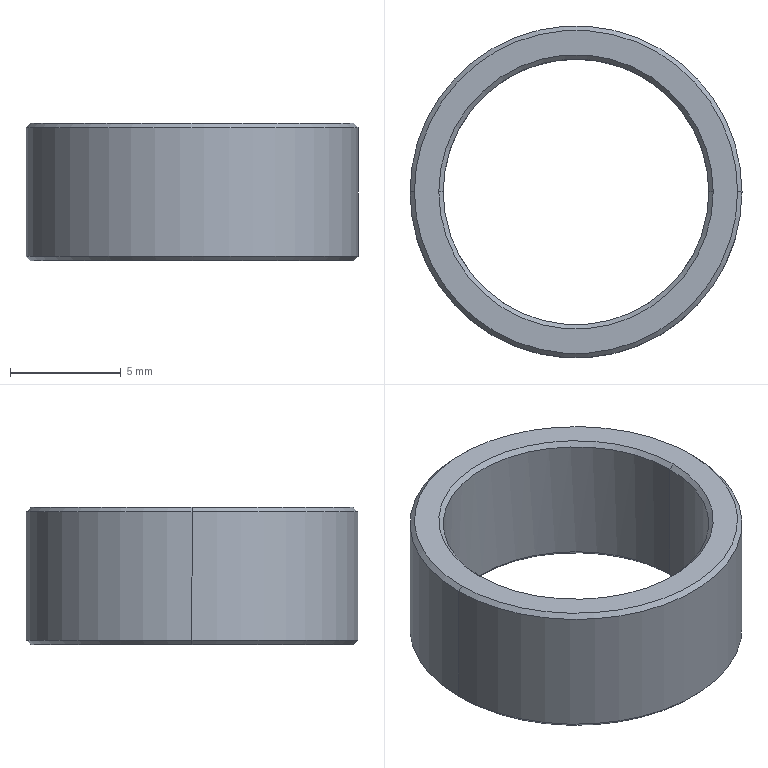Part | STEP file | 0243_002_FWSSM-D15-V12-T6.2 | 1 solid | 14 faces | box 15 x 15 x 6.2 mm | volume 391.034 mm3 | cone 8 | cylinder 4 | plane 2 | commonest cylinder face diameters 12 x2 15 x2
STEP:
#1=CARTESIAN_POINT('',(0.,0.,0.));
#2=DIRECTION('',(0.,0.,1.));
#3=DIRECTION('',(1.,0.,0.));
#4=AXIS2_PLACEMENT_3D('',#1,#2,#3);
#5=CARTESIAN_POINT('',(7.5,0.,-6.));
#6=VERTEX_POINT('',#5);
#7=CARTESIAN_POINT('',(-7.5,0.,-6.));
#8=VERTEX_POINT('',#7);
#9=CARTESIAN_POINT('',(0.,0.,-6.));
#10=DIRECTION('',(0.,0.,1.));
#11=DIRECTION('',(1.,0.,0.));
#12=AXIS2_PLACEMENT_3D('',#9,#10,#11);
#13=CIRCLE('',#12,7.5);
#14=CARTESIAN_POINT('',(0.,0.,-3.1));
#15=DIRECTION('',(0.,0.,1.));
#16=DIRECTION('',(1.,0.,0.));
#17=AXIS2_PLACEMENT_3D('',#14,#15,#16);
#18=CYLINDRICAL_SURFACE('',#17,7.5);
#19=CARTESIAN_POINT('',(0.,-2.9));
#20=DIRECTION('',(1.,0.));
#21=VECTOR('',#20,1.);
#22=LINE('',#19,#21);
#23=(GEOMETRIC_REPRESENTATION_CONTEXT(2)PARAMETRIC_REPRESENTATION_CONTEXT()REPRESENTATION_CONTEXT('',''));
#24=DEFINITIONAL_REPRESENTATION('',(#22),#23);
#25=PCURVE('',#18,#24);
#26=CARTESIAN_POINT('',(0.,0.,-6.));
#27=DIRECTION('',(0.,0.,1.));
#28=DIRECTION('',(1.,0.,0.));
#29=AXIS2_PLACEMENT_3D('',#26,#27,#28);
#30=CONICAL_SURFACE('',#29,7.5,0.7854);
#31=CARTESIAN_POINT('',(0.,0.));
#32=DIRECTION('',(1.,0.));
#33=VECTOR('',#32,1.);
#34=LINE('',#31,#33);
#35=(GEOMETRIC_REPRESENTATION_CONTEXT(2)PARAMETRIC_REPRESENTATION_CONTEXT()REPRESENTATION_CONTEXT('',''));
#36=DEFINITIONAL_REPRESENTATION('',(#34),#35);
#37=PCURVE('',#30,#36);
#38=SURFACE_CURVE('',#13,(#25,#37),.PCURVE_S1.);
#39=EDGE_CURVE('',#6,#8,#38,.T.);
#40=ORIENTED_EDGE('',*,*,#39,.T.);
#41=CARTESIAN_POINT('',(-7.5,0.,-0.2));
#42=VERTEX_POINT('',#41);
#43=CARTESIAN_POINT('',(-7.5,0.,-3.1));
#44=DIRECTION('',(0.,0.,1.));
#45=VECTOR('',#44,1.);
#46=LINE('',#43,#45);
#47=CARTESIAN_POINT('',(3.142,0.));
#48=DIRECTION('',(0.,1.));
#49=VECTOR('',#48,1.);
#50=LINE('',#47,#49);
#51=(GEOMETRIC_REPRESENTATION_CONTEXT(2)PARAMETRIC_REPRESENTATION_CONTEXT()REPRESENTATION_CONTEXT('',''));
#52=DEFINITIONAL_REPRESENTATION('',(#50),#51);
#53=PCURVE('',#18,#52);
#54=CARTESIAN_POINT('',(0.,0.,-3.1));
#55=DIRECTION('',(0.,0.,1.));
#56=DIRECTION('',(1.,0.,0.));
#57=AXIS2_PLACEMENT_3D('',#54,#55,#56);
#58=CYLINDRICAL_SURFACE('',#57,7.5);
#59=CARTESIAN_POINT('',(3.142,0.));
#60=DIRECTION('',(0.,1.));
#61=VECTOR('',#60,1.);
#62=LINE('',#59,#61);
#63=(GEOMETRIC_REPRESENTATION_CONTEXT(2)PARAMETRIC_REPRESENTATION_CONTEXT()REPRESENTATION_CONTEXT('',''));
#64=DEFINITIONAL_REPRESENTATION('',(#62),#63);
#65=PCURVE('',#58,#64);
#66=SURFACE_CURVE('',#46,(#53,#65),.PCURVE_S1.);
#67=EDGE_CURVE('',#8,#42,#66,.T.);
#68=ORIENTED_EDGE('',*,*,#67,.T.);
#69=CARTESIAN_POINT('',(7.5,0.,-0.2));
#70=VERTEX_POINT('',#69);
#71=CARTESIAN_POINT('',(0.,0.,-0.2));
#72=DIRECTION('',(0.,0.,-1.));
#73=DIRECTION('',(1.,0.,0.));
#74=AXIS2_PLACEMENT_3D('',#71,#72,#73);
#75=CIRCLE('',#74,7.5);
#76=CARTESIAN_POINT('',(6.283,2.9));
#77=DIRECTION('',(-1.,0.));
#78=VECTOR('',#77,1.);
#79=LINE('',#76,#78);
#80=(GEOMETRIC_REPRESENTATION_CONTEXT(2)PARAMETRIC_REPRESENTATION_CONTEXT()REPRESENTATION_CONTEXT('',''));
#81=DEFINITIONAL_REPRESENTATION('',(#79),#80);
#82=PCURVE('',#18,#81);
#83=CARTESIAN_POINT('',(0.,0.,-0.2));
#84=DIRECTION('',(0.,0.,-1.));
#85=DIRECTION('',(-1.,0.,0.));
#86=AXIS2_PLACEMENT_3D('',#83,#84,#85);
#87=CONICAL_SURFACE('',#86,7.5,0.7854);
#88=CARTESIAN_POINT('',(-3.142,0.));
#89=DIRECTION('',(1.,0.));
#90=VECTOR('',#89,1.);
#91=LINE('',#88,#90);
#92=(GEOMETRIC_REPRESENTATION_CONTEXT(2)PARAMETRIC_REPRESENTATION_CONTEXT()REPRESENTATION_CONTEXT('',''));
#93=DEFINITIONAL_REPRESENTATION('',(#91),#92);
#94=PCURVE('',#87,#93);
#95=SURFACE_CURVE('',#75,(#82,#94),.PCURVE_S1.);
#96=EDGE_CURVE('',#42,#70,#95,.T.);
#97=ORIENTED_EDGE('',*,*,#96,.T.);
#98=CARTESIAN_POINT('',(7.5,0.,-3.1));
#99=DIRECTION('',(0.,0.,1.));
#100=VECTOR('',#99,1.);
#101=LINE('',#98,#100);
#102=CARTESIAN_POINT('',(0.,0.));
#103=DIRECTION('',(0.,1.));
#104=VECTOR('',#103,1.);
#105=LINE('',#102,#104);
#106=(GEOMETRIC_REPRESENTATION_CONTEXT(2)PARAMETRIC_REPRESENTATION_CONTEXT()REPRESENTATION_CONTEXT('',''));
#107=DEFINITIONAL_REPRESENTATION('',(#105),#106);
#108=PCURVE('',#18,#107);
#109=CARTESIAN_POINT('',(6.283,0.));
#110=DIRECTION('',(0.,1.));
#111=VECTOR('',#110,1.);
#112=LINE('',#109,#111);
#113=(GEOMETRIC_REPRESENTATION_CONTEXT(2)PARAMETRIC_REPRESENTATION_CONTEXT()REPRESENTATION_CONTEXT('',''));
#114=DEFINITIONAL_REPRESENTATION('',(#112),#113);
#115=PCURVE('',#58,#114);
#116=SURFACE_CURVE('',#101,(#108,#115),.PCURVE_S1.);
#117=EDGE_CURVE('',#6,#70,#116,.T.);
#118=ORIENTED_EDGE('',*,*,#117,.F.);
#119=EDGE_LOOP('',(#40,#68,#97,#118));
#120=FACE_BOUND('',#119,.T.);
#121=ADVANCED_FACE('',(#120),#18,.T.);
#122=CARTESIAN_POINT('',(7.3,0.,-6.2));
#123=VERTEX_POINT('',#122);
#124=CARTESIAN_POINT('',(-7.3,0.,-6.2));
#125=VERTEX_POINT('',#124);
#126=CARTESIAN_POINT('',(0.,0.,-6.2));
#127=DIRECTION('',(0.,0.,1.));
#128=DIRECTION('',(1.,0.,0.));
#129=AXIS2_PLACEMENT_3D('',#126,#127,#128);
#130=CIRCLE('',#129,7.3);
#131=CARTESIAN_POINT('',(0.,-0.2));
#132=DIRECTION('',(1.,0.));
#133=VECTOR('',#132,1.);
#134=LINE('',#131,#133);
#135=(GEOMETRIC_REPRESENTATION_CONTEXT(2)PARAMETRIC_REPRESENTATION_CONTEXT()REPRESENTATION_CONTEXT('',''));
#136=DEFINITIONAL_REPRESENTATION('',(#134),#135);
#137=PCURVE('',#30,#136);
#138=CARTESIAN_POINT('',(3.65,0.,-6.2));
#139=DIRECTION('',(0.,0.,-1.));
#140=DIRECTION('',(-1.,0.,0.));
#141=AXIS2_PLACEMENT_3D('',#138,#139,#140);
#142=PLANE('',#141);
#143=CARTESIAN_POINT('',(-3.65,0.));
#144=CARTESIAN_POINT('',(-3.65,12.644));
#145=CARTESIAN_POINT('',(7.3,6.322));
#146=CARTESIAN_POINT('',(18.25,0.));
#147=CARTESIAN_POINT('',(7.3,-6.322));
#148=CARTESIAN_POINT('',(-3.65,-12.644));
#149=CARTESIAN_POINT('',(-3.65,0.));
#150=(BOUNDED_CURVE()B_SPLINE_CURVE(2,(#143,#144,#145,#146,#147,#148,#149),.UNSPECIFIED.,.T.,.F.)B_SPLINE_CURVE_WITH_KNOTS((1,2,2,2,2,1),(-2.094,0.,2.094,4.189,6.283,8.378),.UNSPECIFIED.)CURVE()GEOMETRIC_REPRESENTATION_ITEM()RATIONAL_B_SPLINE_CURVE((1.,0.5,1.,0.5,1.,0.5,1.))REPRESENTATION_ITEM(''));
#151=(GEOMETRIC_REPRESENTATION_CONTEXT(2)PARAMETRIC_REPRESENTATION_CONTEXT()REPRESENTATION_CONTEXT('',''));
#152=DEFINITIONAL_REPRESENTATION('',(#150),#151);
#153=PCURVE('',#142,#152);
#154=SURFACE_CURVE('',#130,(#137,#153),.PCURVE_S1.);
#155=EDGE_CURVE('',#123,#125,#154,.T.);
#156=ORIENTED_EDGE('',*,*,#155,.T.);
#157=CARTESIAN_POINT('',(-7.5,0.,-6.));
#158=DIRECTION('',(-0.7071,0.,0.7071));
#159=VECTOR('',#158,1.);
#160=LINE('',#157,#159);
#161=CARTESIAN_POINT('',(3.142,0.));
#162=DIRECTION('',(0.,1.));
#163=VECTOR('',#162,1.);
#164=LINE('',#161,#163);
#165=(GEOMETRIC_REPRESENTATION_CONTEXT(2)PARAMETRIC_REPRESENTATION_CONTEXT()REPRESENTATION_CONTEXT('',''));
#166=DEFINITIONAL_REPRESENTATION('',(#164),#165);
#167=PCURVE('',#30,#166);
#168=CARTESIAN_POINT('',(0.,0.,-6.));
#169=DIRECTION('',(0.,0.,1.));
#170=DIRECTION('',(1.,0.,0.));
#171=AXIS2_PLACEMENT_3D('',#168,#169,#170);
#172=CONICAL_SURFACE('',#171,7.5,0.7854);
#173=CARTESIAN_POINT('',(3.142,0.));
#174=DIRECTION('',(0.,1.));
#175=VECTOR('',#174,1.);
#176=LINE('',#173,#175);
#177=(GEOMETRIC_REPRESENTATION_CONTEXT(2)PARAMETRIC_REPRESENTATION_CONTEXT()REPRESENTATION_CONTEXT('',''));
#178=DEFINITIONAL_REPRESENTATION('',(#176),#177);
#179=PCURVE('',#172,#178);
#180=SURFACE_CURVE('',#160,(#167,#179),.PCURVE_S1.);
#181=EDGE_CURVE('',#125,#8,#180,.T.);
#182=ORIENTED_EDGE('',*,*,#181,.T.);
#183=ORIENTED_EDGE('',*,*,#39,.F.);
#184=CARTESIAN_POINT('',(7.5,0.,-6.));
#185=DIRECTION('',(0.7071,0.,0.7071));
#186=VECTOR('',#185,1.);
#187=LINE('',#184,#186);
#188=CARTESIAN_POINT('',(0.,0.));
#189=DIRECTION('',(0.,1.));
#190=VECTOR('',#189,1.);
#191=LINE('',#188,#190);
#192=(GEOMETRIC_REPRESENTATION_CONTEXT(2)PARAMETRIC_REPRESENTATION_CONTEXT()REPRESENTATION_CONTEXT('',''));
#193=DEFINITIONAL_REPRESENTATION('',(#191),#192);
#194=PCURVE('',#30,#193);
#195=CARTESIAN_POINT('',(6.283,0.));
#196=DIRECTION('',(0.,1.));
#197=VECTOR('',#196,1.);
#198=LINE('',#195,#197);
#199=(GEOMETRIC_REPRESENTATION_CONTEXT(2)PARAMETRIC_REPRESENTATION_CONTEXT()REPRESENTATION_CONTEXT('',''));
#200=DEFINITIONAL_REPRESENTATION('',(#198),#199);
#201=PCURVE('',#172,#200);
#202=SURFACE_CURVE('',#187,(#194,#201),.PCURVE_S1.);
#203=EDGE_CURVE('',#123,#6,#202,.T.);
#204=ORIENTED_EDGE('',*,*,#203,.F.);
#205=EDGE_LOOP('',(#156,#182,#183,#204));
#206=FACE_BOUND('',#205,.T.);
#207=ADVANCED_FACE('',(#206),#30,.T.);
#208=CARTESIAN_POINT('',(-7.3,0.,0.));
#209=VERTEX_POINT('',#208);
#210=CARTESIAN_POINT('',(7.3,0.,0.));
#211=VERTEX_POINT('',#210);
#212=CARTESIAN_POINT('',(0.,0.,0.));
#213=DIRECTION('',(0.,0.,-1.));
#214=DIRECTION('',(-1.,0.,0.));
#215=AXIS2_PLACEMENT_3D('',#212,#213,#214);
#216=CIRCLE('',#215,7.3);
#217=CARTESIAN_POINT('',(0.,-0.2));
#218=DIRECTION('',(1.,0.));
#219=VECTOR('',#218,1.);
#220=LINE('',#217,#219);
#221=(GEOMETRIC_REPRESENTATION_CONTEXT(2)PARAMETRIC_REPRESENTATION_CONTEXT()REPRESENTATION_CONTEXT('',''));
#222=DEFINITIONAL_REPRESENTATION('',(#220),#221);
#223=PCURVE('',#87,#222);
#224=CARTESIAN_POINT('',(3.65,0.,0.));
#225=DIRECTION('',(0.,0.,1.));
#226=DIRECTION('',(1.,0.,0.));
#227=AXIS2_PLACEMENT_3D('',#224,#225,#226);
#228=PLANE('',#227);
#229=CARTESIAN_POINT('',(-10.95,0.));
#230=CARTESIAN_POINT('',(-10.95,12.644));
#231=CARTESIAN_POINT('',(0.,6.322));
#232=CARTESIAN_POINT('',(10.95,0.));
#233=CARTESIAN_POINT('',(0.,-6.322));
#234=CARTESIAN_POINT('',(-10.95,-12.644));
#235=CARTESIAN_POINT('',(-10.95,0.));
#236=(BOUNDED_CURVE()B_SPLINE_CURVE(2,(#229,#230,#231,#232,#233,#234,#235),.UNSPECIFIED.,.T.,.F.)B_SPLINE_CURVE_WITH_KNOTS((1,2,2,2,2,1),(-2.094,0.,2.094,4.189,6.283,8.378),.UNSPECIFIED.)CURVE()GEOMETRIC_REPRESENTATION_ITEM()RATIONAL_B_SPLINE_CURVE((1.,0.5,1.,0.5,1.,0.5,1.))REPRESENTATION_ITEM(''));
#237=(GEOMETRIC_REPRESENTATION_CONTEXT(2)PARAMETRIC_REPRESENTATION_CONTEXT()REPRESENTATION_CONTEXT('',''));
#238=DEFINITIONAL_REPRESENTATION('',(#236),#237);
#239=PCURVE('',#228,#238);
#240=SURFACE_CURVE('',#216,(#223,#239),.PCURVE_S1.);
#241=EDGE_CURVE('',#209,#211,#240,.T.);
#242=ORIENTED_EDGE('',*,*,#241,.T.);
#243=CARTESIAN_POINT('',(7.5,0.,-0.2));
#244=DIRECTION('',(0.7071,0.,-0.7071));
#245=VECTOR('',#244,1.);
#246=LINE('',#243,#245);
#247=CARTESIAN_POINT('',(3.142,0.));
#248=DIRECTION('',(0.,1.));
#249=VECTOR('',#248,1.);
#250=LINE('',#247,#249);
#251=(GEOMETRIC_REPRESENTATION_CONTEXT(2)PARAMETRIC_REPRESENTATION_CONTEXT()REPRESENTATION_CONTEXT('',''));
#252=DEFINITIONAL_REPRESENTATION('',(#250),#251);
#253=PCURVE('',#87,#252);
#254=CARTESIAN_POINT('',(0.,0.,-0.2));
#255=DIRECTION('',(0.,0.,-1.));
#256=DIRECTION('',(-1.,0.,0.));
#257=AXIS2_PLACEMENT_3D('',#254,#255,#256);
#258=CONICAL_SURFACE('',#257,7.5,0.7854);
#259=CARTESIAN_POINT('',(3.142,0.));
#260=DIRECTION('',(0.,1.));
#261=VECTOR('',#260,1.);
#262=LINE('',#259,#261);
#263=(GEOMETRIC_REPRESENTATION_CONTEXT(2)PARAMETRIC_REPRESENTATION_CONTEXT()REPRESENTATION_CONTEXT('',''));
#264=DEFINITIONAL_REPRESENTATION('',(#262),#263);
#265=PCURVE('',#258,#264);
#266=SURFACE_CURVE('',#246,(#253,#265),.PCURVE_S1.);
#267=EDGE_CURVE('',#211,#70,#266,.T.);
#268=ORIENTED_EDGE('',*,*,#267,.T.);
#269=ORIENTED_EDGE('',*,*,#96,.F.);
#270=CARTESIAN_POINT('',(-7.5,0.,-0.2));
#271=DIRECTION('',(-0.7071,0.,-0.7071));
#272=VECTOR('',#271,1.);
#273=LINE('',#270,#272);
#274=CARTESIAN_POINT('',(0.,0.));
#275=DIRECTION('',(0.,1.));
#276=VECTOR('',#275,1.);
#277=LINE('',#274,#276);
#278=(GEOMETRIC_REPRESENTATION_CONTEXT(2)PARAMETRIC_REPRESENTATION_CONTEXT()REPRESENTATION_CONTEXT('',''));
#279=DEFINITIONAL_REPRESENTATION('',(#277),#278);
#280=PCURVE('',#87,#279);
#281=CARTESIAN_POINT('',(6.283,0.));
#282=DIRECTION('',(0.,1.));
#283=VECTOR('',#282,1.);
#284=LINE('',#281,#283);
#285=(GEOMETRIC_REPRESENTATION_CONTEXT(2)PARAMETRIC_REPRESENTATION_CONTEXT()REPRESENTATION_CONTEXT('',''));
#286=DEFINITIONAL_REPRESENTATION('',(#284),#285);
#287=PCURVE('',#258,#286);
#288=SURFACE_CURVE('',#273,(#280,#287),.PCURVE_S1.);
#289=EDGE_CURVE('',#209,#42,#288,.T.);
#290=ORIENTED_EDGE('',*,*,#289,.F.);
#291=EDGE_LOOP('',(#242,#268,#269,#290));
#292=FACE_BOUND('',#291,.T.);
#293=ADVANCED_FACE('',(#292),#87,.T.);
#294=CARTESIAN_POINT('',(-6.,0.,-6.));
#295=VERTEX_POINT('',#294);
#296=CARTESIAN_POINT('',(0.,6.,-6.));
#297=VERTEX_POINT('',#296);
#298=CARTESIAN_POINT('',(0.,0.,-6.));
#299=DIRECTION('',(0.,0.,-1.));
#300=DIRECTION('',(1.,0.,0.));
#301=AXIS2_PLACEMENT_3D('',#298,#299,#300);
#302=CIRCLE('',#301,6.);
#303=CARTESIAN_POINT('',(0.,0.,-6.2));
#304=DIRECTION('',(0.,0.,-1.));
#305=DIRECTION('',(0.,1.,0.));
#306=AXIS2_PLACEMENT_3D('',#303,#304,#305);
#307=CONICAL_SURFACE('',#306,6.2,0.7854);
#308=CARTESIAN_POINT('',(1.571,-0.2));
#309=DIRECTION('',(1.,0.));
#310=VECTOR('',#309,1.);
#311=LINE('',#308,#310);
#312=(GEOMETRIC_REPRESENTATION_CONTEXT(2)PARAMETRIC_REPRESENTATION_CONTEXT()REPRESENTATION_CONTEXT('',''));
#313=DEFINITIONAL_REPRESENTATION('',(#311),#312);
#314=PCURVE('',#307,#313);
#315=CARTESIAN_POINT('',(0.,0.,-3.1));
#316=DIRECTION('',(0.,0.,1.));
#317=DIRECTION('',(1.,0.,0.));
#318=AXIS2_PLACEMENT_3D('',#315,#316,#317);
#319=CYLINDRICAL_SURFACE('',#318,6.);
#320=CARTESIAN_POINT('',(6.283,-2.9));
#321=DIRECTION('',(-1.,0.));
#322=VECTOR('',#321,1.);
#323=LINE('',#320,#322);
#324=(GEOMETRIC_REPRESENTATION_CONTEXT(2)PARAMETRIC_REPRESENTATION_CONTEXT()REPRESENTATION_CONTEXT('',''));
#325=DEFINITIONAL_REPRESENTATION('',(#323),#324);
#326=PCURVE('',#319,#325);
#327=SURFACE_CURVE('',#302,(#314,#326),.PCURVE_S1.);
#328=EDGE_CURVE('',#295,#297,#327,.T.);
#329=ORIENTED_EDGE('',*,*,#328,.T.);
#330=CARTESIAN_POINT('',(0.,6.2,-6.2));
#331=VERTEX_POINT('',#330);
#332=CARTESIAN_POINT('',(0.,6.2,-6.2));
#333=DIRECTION('',(0.,0.7071,-0.7071));
#334=VECTOR('',#333,1.);
#335=LINE('',#332,#334);
#336=CARTESIAN_POINT('',(6.283,0.));
#337=DIRECTION('',(0.,1.));
#338=VECTOR('',#337,1.);
#339=LINE('',#336,#338);
#340=(GEOMETRIC_REPRESENTATION_CONTEXT(2)PARAMETRIC_REPRESENTATION_CONTEXT()REPRESENTATION_CONTEXT('',''));
#341=DEFINITIONAL_REPRESENTATION('',(#339),#340);
#342=PCURVE('',#307,#341);
#343=CARTESIAN_POINT('',(0.,0.,-6.2));
#344=DIRECTION('',(0.,0.,-1.));
#345=DIRECTION('',(0.,1.,0.));
#346=AXIS2_PLACEMENT_3D('',#343,#344,#345);
#347=CONICAL_SURFACE('',#346,6.2,0.7854);
#348=CARTESIAN_POINT('',(0.,0.));
#349=DIRECTION('',(0.,1.));
#350=VECTOR('',#349,1.);
#351=LINE('',#348,#350);
#352=(GEOMETRIC_REPRESENTATION_CONTEXT(2)PARAMETRIC_REPRESENTATION_CONTEXT()REPRESENTATION_CONTEXT('',''));
#353=DEFINITIONAL_REPRESENTATION('',(#351),#352);
#354=PCURVE('',#347,#353);
#355=SURFACE_CURVE('',#335,(#342,#354),.PCURVE_S1.);
#356=EDGE_CURVE('',#297,#331,#355,.T.);
#357=ORIENTED_EDGE('',*,*,#356,.T.);
#358=CARTESIAN_POINT('',(0.,-6.2,-6.2));
#359=VERTEX_POINT('',#358);
#360=CARTESIAN_POINT('',(0.,0.,-6.2));
#361=DIRECTION('',(0.,0.,1.));
#362=DIRECTION('',(0.,1.,0.));
#363=AXIS2_PLACEMENT_3D('',#360,#361,#362);
#364=CIRCLE('',#363,6.2);
#365=CARTESIAN_POINT('',(6.283,0.));
#366=DIRECTION('',(-1.,0.));
#367=VECTOR('',#366,1.);
#368=LINE('',#365,#367);
#369=(GEOMETRIC_REPRESENTATION_CONTEXT(2)PARAMETRIC_REPRESENTATION_CONTEXT()REPRESENTATION_CONTEXT('',''));
#370=DEFINITIONAL_REPRESENTATION('',(#368),#369);
#371=PCURVE('',#307,#370);
#372=CARTESIAN_POINT('',(3.65,6.2));
#373=CARTESIAN_POINT('',(14.389,6.2));
#374=CARTESIAN_POINT('',(9.019,-3.1));
#375=CARTESIAN_POINT('',(3.65,-12.4));
#376=CARTESIAN_POINT('',(-1.719,-3.1));
#377=CARTESIAN_POINT('',(-7.089,6.2));
#378=CARTESIAN_POINT('',(3.65,6.2));
#379=(BOUNDED_CURVE()B_SPLINE_CURVE(2,(#372,#373,#374,#375,#376,#377,#378),.UNSPECIFIED.,.T.,.F.)B_SPLINE_CURVE_WITH_KNOTS((1,2,2,2,2,1),(-2.094,0.,2.094,4.189,6.283,8.378),.UNSPECIFIED.)CURVE()GEOMETRIC_REPRESENTATION_ITEM()RATIONAL_B_SPLINE_CURVE((1.,0.5,1.,0.5,1.,0.5,1.))REPRESENTATION_ITEM(''));
#380=(GEOMETRIC_REPRESENTATION_CONTEXT(2)PARAMETRIC_REPRESENTATION_CONTEXT()REPRESENTATION_CONTEXT('',''));
#381=DEFINITIONAL_REPRESENTATION('',(#379),#380);
#382=PCURVE('',#142,#381);
#383=SURFACE_CURVE('',#364,(#371,#382),.PCURVE_S1.);
#384=EDGE_CURVE('',#331,#359,#383,.T.);
#385=ORIENTED_EDGE('',*,*,#384,.T.);
#386=CARTESIAN_POINT('',(0.,-6.,-6.));
#387=VERTEX_POINT('',#386);
#388=CARTESIAN_POINT('',(0.,-6.2,-6.2));
#389=DIRECTION('',(0.,-0.7071,-0.7071));
#390=VECTOR('',#389,1.);
#391=LINE('',#388,#390);
#392=CARTESIAN_POINT('',(3.142,0.));
#393=DIRECTION('',(0.,1.));
#394=VECTOR('',#393,1.);
#395=LINE('',#392,#394);
#396=(GEOMETRIC_REPRESENTATION_CONTEXT(2)PARAMETRIC_REPRESENTATION_CONTEXT()REPRESENTATION_CONTEXT('',''));
#397=DEFINITIONAL_REPRESENTATION('',(#395),#396);
#398=PCURVE('',#307,#397);
#399=CARTESIAN_POINT('',(3.142,0.));
#400=DIRECTION('',(0.,1.));
#401=VECTOR('',#400,1.);
#402=LINE('',#399,#401);
#403=(GEOMETRIC_REPRESENTATION_CONTEXT(2)PARAMETRIC_REPRESENTATION_CONTEXT()REPRESENTATION_CONTEXT('',''));
#404=DEFINITIONAL_REPRESENTATION('',(#402),#403);
#405=PCURVE('',#347,#404);
#406=SURFACE_CURVE('',#391,(#398,#405),.PCURVE_S1.);
#407=EDGE_CURVE('',#387,#359,#406,.T.);
#408=ORIENTED_EDGE('',*,*,#407,.F.);
#409=CARTESIAN_POINT('',(0.,0.,-6.));
#410=DIRECTION('',(0.,0.,-1.));
#411=DIRECTION('',(1.,0.,0.));
#412=AXIS2_PLACEMENT_3D('',#409,#410,#411);
#413=CIRCLE('',#412,6.);
#414=CARTESIAN_POINT('',(1.571,-0.2));
#415=DIRECTION('',(1.,0.));
#416=VECTOR('',#415,1.);
#417=LINE('',#414,#416);
#418=(GEOMETRIC_REPRESENTATION_CONTEXT(2)PARAMETRIC_REPRESENTATION_CONTEXT()REPRESENTATION_CONTEXT('',''));
#419=DEFINITIONAL_REPRESENTATION('',(#417),#418);
#420=PCURVE('',#307,#419);
#421=CARTESIAN_POINT('',(0.,0.,-3.1));
#422=DIRECTION('',(0.,0.,1.));
#423=DIRECTION('',(1.,0.,0.));
#424=AXIS2_PLACEMENT_3D('',#421,#422,#423);
#425=CYLINDRICAL_SURFACE('',#424,6.);
#426=CARTESIAN_POINT('',(6.283,-2.9));
#427=DIRECTION('',(-1.,0.));
#428=VECTOR('',#427,1.);
#429=LINE('',#426,#428);
#430=(GEOMETRIC_REPRESENTATION_CONTEXT(2)PARAMETRIC_REPRESENTATION_CONTEXT()REPRESENTATION_CONTEXT('',''));
#431=DEFINITIONAL_REPRESENTATION('',(#429),#430);
#432=PCURVE('',#425,#431);
#433=SURFACE_CURVE('',#413,(#420,#432),.PCURVE_S1.);
#434=EDGE_CURVE('',#387,#295,#433,.T.);
#435=ORIENTED_EDGE('',*,*,#434,.T.);
#436=EDGE_LOOP('',(#329,#357,#385,#408,#435));
#437=FACE_BOUND('',#436,.F.);
#438=ADVANCED_FACE('',(#437),#307,.F.);
#439=CARTESIAN_POINT('',(6.,0.,-0.2));
#440=VERTEX_POINT('',#439);
#441=CARTESIAN_POINT('',(6.2,0.,0.));
#442=VERTEX_POINT('',#441);
#443=CARTESIAN_POINT('',(6.2,0.,0.));
#444=DIRECTION('',(0.7071,0.,0.7071));
#445=VECTOR('',#444,1.);
#446=LINE('',#443,#445);
#447=CARTESIAN_POINT('',(0.,0.,0.));
#448=DIRECTION('',(0.,0.,1.));
#449=DIRECTION('',(1.,0.,0.));
#450=AXIS2_PLACEMENT_3D('',#447,#448,#449);
#451=CONICAL_SURFACE('',#450,6.2,0.7854);
#452=CARTESIAN_POINT('',(6.283,0.));
#453=DIRECTION('',(0.,1.));
#454=VECTOR('',#453,1.);
#455=LINE('',#452,#454);
#456=(GEOMETRIC_REPRESENTATION_CONTEXT(2)PARAMETRIC_REPRESENTATION_CONTEXT()REPRESENTATION_CONTEXT('',''));
#457=DEFINITIONAL_REPRESENTATION('',(#455),#456);
#458=PCURVE('',#451,#457);
#459=CARTESIAN_POINT('',(0.,0.,0.));
#460=DIRECTION('',(0.,0.,1.));
#461=DIRECTION('',(1.,0.,0.));
#462=AXIS2_PLACEMENT_3D('',#459,#460,#461);
#463=CONICAL_SURFACE('',#462,6.2,0.7854);
#464=CARTESIAN_POINT('',(0.,0.));
#465=DIRECTION('',(0.,1.));
#466=VECTOR('',#465,1.);
#467=LINE('',#464,#466);
#468=(GEOMETRIC_REPRESENTATION_CONTEXT(2)PARAMETRIC_REPRESENTATION_CONTEXT()REPRESENTATION_CONTEXT('',''));
#469=DEFINITIONAL_REPRESENTATION('',(#467),#468);
#470=PCURVE('',#463,#469);
#471=SURFACE_CURVE('',#446,(#458,#470),.PCURVE_S1.);
#472=EDGE_CURVE('',#440,#442,#471,.T.);
#473=ORIENTED_EDGE('',*,*,#472,.T.);
#474=CARTESIAN_POINT('',(-6.2,0.,0.));
#475=VERTEX_POINT('',#474);
#476=CARTESIAN_POINT('',(0.,0.,0.));
#477=DIRECTION('',(0.,0.,-1.));
#478=DIRECTION('',(1.,0.,0.));
#479=AXIS2_PLACEMENT_3D('',#476,#477,#478);
#480=CIRCLE('',#479,6.2);
#481=CARTESIAN_POINT('',(6.283,0.));
#482=DIRECTION('',(-1.,0.));
#483=VECTOR('',#482,1.);
#484=LINE('',#481,#483);
#485=(GEOMETRIC_REPRESENTATION_CONTEXT(2)PARAMETRIC_REPRESENTATION_CONTEXT()REPRESENTATION_CONTEXT('',''));
#486=DEFINITIONAL_REPRESENTATION('',(#484),#485);
#487=PCURVE('',#451,#486);
#488=CARTESIAN_POINT('',(2.55,0.));
#489=CARTESIAN_POINT('',(2.55,-10.739));
#490=CARTESIAN_POINT('',(-6.75,-5.369));
#491=CARTESIAN_POINT('',(-16.05,0.));
#492=CARTESIAN_POINT('',(-6.75,5.369));
#493=CARTESIAN_POINT('',(2.55,10.739));
#494=CARTESIAN_POINT('',(2.55,0.));
#495=(BOUNDED_CURVE()B_SPLINE_CURVE(2,(#488,#489,#490,#491,#492,#493,#494),.UNSPECIFIED.,.T.,.F.)B_SPLINE_CURVE_WITH_KNOTS((1,2,2,2,2,1),(-2.094,0.,2.094,4.189,6.283,8.378),.UNSPECIFIED.)CURVE()GEOMETRIC_REPRESENTATION_ITEM()RATIONAL_B_SPLINE_CURVE((1.,0.5,1.,0.5,1.,0.5,1.))REPRESENTATION_ITEM(''));
#496=(GEOMETRIC_REPRESENTATION_CONTEXT(2)PARAMETRIC_REPRESENTATION_CONTEXT()REPRESENTATION_CONTEXT('',''));
#497=DEFINITIONAL_REPRESENTATION('',(#495),#496);
#498=PCURVE('',#228,#497);
#499=SURFACE_CURVE('',#480,(#487,#498),.PCURVE_S1.);
#500=EDGE_CURVE('',#442,#475,#499,.T.);
#501=ORIENTED_EDGE('',*,*,#500,.T.);
#502=CARTESIAN_POINT('',(-6.,0.,-0.2));
#503=VERTEX_POINT('',#502);
#504=CARTESIAN_POINT('',(-6.2,0.,0.));
#505=DIRECTION('',(-0.7071,0.,0.7071));
#506=VECTOR('',#505,1.);
#507=LINE('',#504,#506);
#508=CARTESIAN_POINT('',(3.142,0.));
#509=DIRECTION('',(0.,1.));
#510=VECTOR('',#509,1.);
#511=LINE('',#508,#510);
#512=(GEOMETRIC_REPRESENTATION_CONTEXT(2)PARAMETRIC_REPRESENTATION_CONTEXT()REPRESENTATION_CONTEXT('',''));
#513=DEFINITIONAL_REPRESENTATION('',(#511),#512);
#514=PCURVE('',#451,#513);
#515=CARTESIAN_POINT('',(3.142,0.));
#516=DIRECTION('',(0.,1.));
#517=VECTOR('',#516,1.);
#518=LINE('',#515,#517);
#519=(GEOMETRIC_REPRESENTATION_CONTEXT(2)PARAMETRIC_REPRESENTATION_CONTEXT()REPRESENTATION_CONTEXT('',''));
#520=DEFINITIONAL_REPRESENTATION('',(#518),#519);
#521=PCURVE('',#463,#520);
#522=SURFACE_CURVE('',#507,(#514,#521),.PCURVE_S1.);
#523=EDGE_CURVE('',#503,#475,#522,.T.);
#524=ORIENTED_EDGE('',*,*,#523,.F.);
#525=CARTESIAN_POINT('',(0.,0.,-0.2));
#526=DIRECTION('',(0.,0.,1.));
#527=DIRECTION('',(1.,0.,0.));
#528=AXIS2_PLACEMENT_3D('',#525,#526,#527);
#529=CIRCLE('',#528,6.);
#530=CARTESIAN_POINT('',(0.,-0.2));
#531=DIRECTION('',(1.,0.));
#532=VECTOR('',#531,1.);
#533=LINE('',#530,#532);
#534=(GEOMETRIC_REPRESENTATION_CONTEXT(2)PARAMETRIC_REPRESENTATION_CONTEXT()REPRESENTATION_CONTEXT('',''));
#535=DEFINITIONAL_REPRESENTATION('',(#533),#534);
#536=PCURVE('',#451,#535);
#537=CARTESIAN_POINT('',(0.,2.9));
#538=DIRECTION('',(1.,0.));
#539=VECTOR('',#538,1.);
#540=LINE('',#537,#539);
#541=(GEOMETRIC_REPRESENTATION_CONTEXT(2)PARAMETRIC_REPRESENTATION_CONTEXT()REPRESENTATION_CONTEXT('',''));
#542=DEFINITIONAL_REPRESENTATION('',(#540),#541);
#543=PCURVE('',#425,#542);
#544=SURFACE_CURVE('',#529,(#536,#543),.PCURVE_S1.);
#545=EDGE_CURVE('',#503,#440,#544,.T.);
#546=ORIENTED_EDGE('',*,*,#545,.T.);
#547=EDGE_LOOP('',(#473,#501,#524,#546));
#548=FACE_BOUND('',#547,.F.);
#549=ADVANCED_FACE('',(#548),#451,.F.);
#550=CARTESIAN_POINT('',(6.,0.,-6.));
#551=VERTEX_POINT('',#550);
#552=CARTESIAN_POINT('',(6.,0.,-3.1));
#553=DIRECTION('',(0.,0.,1.));
#554=VECTOR('',#553,1.);
#555=LINE('',#552,#554);
#556=CARTESIAN_POINT('',(6.283,0.));
#557=DIRECTION('',(0.,1.));
#558=VECTOR('',#557,1.);
#559=LINE('',#556,#558);
#560=(GEOMETRIC_REPRESENTATION_CONTEXT(2)PARAMETRIC_REPRESENTATION_CONTEXT()REPRESENTATION_CONTEXT('',''));
#561=DEFINITIONAL_REPRESENTATION('',(#559),#560);
#562=PCURVE('',#425,#561);
#563=CARTESIAN_POINT('',(0.,0.));
#564=DIRECTION('',(0.,1.));
#565=VECTOR('',#564,1.);
#566=LINE('',#563,#565);
#567=(GEOMETRIC_REPRESENTATION_CONTEXT(2)PARAMETRIC_REPRESENTATION_CONTEXT()REPRESENTATION_CONTEXT('',''));
#568=DEFINITIONAL_REPRESENTATION('',(#566),#567);
#569=PCURVE('',#319,#568);
#570=SURFACE_CURVE('',#555,(#562,#569),.PCURVE_S1.);
#571=EDGE_CURVE('',#551,#440,#570,.T.);
#572=ORIENTED_EDGE('',*,*,#571,.T.);
#573=ORIENTED_EDGE('',*,*,#545,.F.);
#574=CARTESIAN_POINT('',(-6.,0.,-3.1));
#575=DIRECTION('',(0.,0.,1.));
#576=VECTOR('',#575,1.);
#577=LINE('',#574,#576);
#578=CARTESIAN_POINT('',(3.142,0.));
#579=DIRECTION('',(0.,1.));
#580=VECTOR('',#579,1.);
#581=LINE('',#578,#580);
#582=(GEOMETRIC_REPRESENTATION_CONTEXT(2)PARAMETRIC_REPRESENTATION_CONTEXT()REPRESENTATION_CONTEXT('',''));
#583=DEFINITIONAL_REPRESENTATION('',(#581),#582);
#584=PCURVE('',#425,#583);
#585=CARTESIAN_POINT('',(3.142,0.));
#586=DIRECTION('',(0.,1.));
#587=VECTOR('',#586,1.);
#588=LINE('',#585,#587);
#589=(GEOMETRIC_REPRESENTATION_CONTEXT(2)PARAMETRIC_REPRESENTATION_CONTEXT()REPRESENTATION_CONTEXT('',''));
#590=DEFINITIONAL_REPRESENTATION('',(#588),#589);
#591=PCURVE('',#319,#590);
#592=SURFACE_CURVE('',#577,(#584,#591),.PCURVE_S1.);
#593=EDGE_CURVE('',#295,#503,#592,.T.);
#594=ORIENTED_EDGE('',*,*,#593,.F.);
#595=ORIENTED_EDGE('',*,*,#434,.F.);
#596=CARTESIAN_POINT('',(0.,0.,-6.));
#597=DIRECTION('',(0.,0.,-1.));
#598=DIRECTION('',(1.,0.,0.));
#599=AXIS2_PLACEMENT_3D('',#596,#597,#598);
#600=CIRCLE('',#599,6.);
#601=CARTESIAN_POINT('',(6.283,-2.9));
#602=DIRECTION('',(-1.,0.));
#603=VECTOR('',#602,1.);
#604=LINE('',#601,#603);
#605=(GEOMETRIC_REPRESENTATION_CONTEXT(2)PARAMETRIC_REPRESENTATION_CONTEXT()REPRESENTATION_CONTEXT('',''));
#606=DEFINITIONAL_REPRESENTATION('',(#604),#605);
#607=PCURVE('',#425,#606);
#608=CARTESIAN_POINT('',(1.571,-0.2));
#609=DIRECTION('',(1.,0.));
#610=VECTOR('',#609,1.);
#611=LINE('',#608,#610);
#612=(GEOMETRIC_REPRESENTATION_CONTEXT(2)PARAMETRIC_REPRESENTATION_CONTEXT()REPRESENTATION_CONTEXT('',''));
#613=DEFINITIONAL_REPRESENTATION('',(#611),#612);
#614=PCURVE('',#347,#613);
#615=SURFACE_CURVE('',#600,(#607,#614),.PCURVE_S1.);
#616=EDGE_CURVE('',#551,#387,#615,.T.);
#617=ORIENTED_EDGE('',*,*,#616,.F.);
#618=EDGE_LOOP('',(#572,#573,#594,#595,#617));
#619=FACE_BOUND('',#618,.F.);
#620=ADVANCED_FACE('',(#619),#425,.F.);
#621=ORIENTED_EDGE('',*,*,#67,.F.);
#622=CARTESIAN_POINT('',(0.,0.,-6.));
#623=DIRECTION('',(0.,0.,1.));
#624=DIRECTION('',(1.,0.,0.));
#625=AXIS2_PLACEMENT_3D('',#622,#623,#624);
#626=CIRCLE('',#625,7.5);
#627=CARTESIAN_POINT('',(0.,-2.9));
#628=DIRECTION('',(1.,0.));
#629=VECTOR('',#628,1.);
#630=LINE('',#627,#629);
#631=(GEOMETRIC_REPRESENTATION_CONTEXT(2)PARAMETRIC_REPRESENTATION_CONTEXT()REPRESENTATION_CONTEXT('',''));
#632=DEFINITIONAL_REPRESENTATION('',(#630),#631);
#633=PCURVE('',#58,#632);
#634=CARTESIAN_POINT('',(0.,0.));
#635=DIRECTION('',(1.,0.));
#636=VECTOR('',#635,1.);
#637=LINE('',#634,#636);
#638=(GEOMETRIC_REPRESENTATION_CONTEXT(2)PARAMETRIC_REPRESENTATION_CONTEXT()REPRESENTATION_CONTEXT('',''));
#639=DEFINITIONAL_REPRESENTATION('',(#637),#638);
#640=PCURVE('',#172,#639);
#641=SURFACE_CURVE('',#626,(#633,#640),.PCURVE_S1.);
#642=EDGE_CURVE('',#8,#6,#641,.T.);
#643=ORIENTED_EDGE('',*,*,#642,.T.);
#644=ORIENTED_EDGE('',*,*,#117,.T.);
#645=CARTESIAN_POINT('',(0.,0.,-0.2));
#646=DIRECTION('',(0.,0.,-1.));
#647=DIRECTION('',(1.,0.,0.));
#648=AXIS2_PLACEMENT_3D('',#645,#646,#647);
#649=CIRCLE('',#648,7.5);
#650=CARTESIAN_POINT('',(6.283,2.9));
#651=DIRECTION('',(-1.,0.));
#652=VECTOR('',#651,1.);
#653=LINE('',#650,#652);
#654=(GEOMETRIC_REPRESENTATION_CONTEXT(2)PARAMETRIC_REPRESENTATION_CONTEXT()REPRESENTATION_CONTEXT('',''));
#655=DEFINITIONAL_REPRESENTATION('',(#653),#654);
#656=PCURVE('',#58,#655);
#657=CARTESIAN_POINT('',(3.142,0.));
#658=DIRECTION('',(1.,0.));
#659=VECTOR('',#658,1.);
#660=LINE('',#657,#659);
#661=(GEOMETRIC_REPRESENTATION_CONTEXT(2)PARAMETRIC_REPRESENTATION_CONTEXT()REPRESENTATION_CONTEXT('',''));
#662=DEFINITIONAL_REPRESENTATION('',(#660),#661);
#663=PCURVE('',#258,#662);
#664=SURFACE_CURVE('',#649,(#656,#663),.PCURVE_S1.);
#665=EDGE_CURVE('',#70,#42,#664,.T.);
#666=ORIENTED_EDGE('',*,*,#665,.T.);
#667=EDGE_LOOP('',(#621,#643,#644,#666));
#668=FACE_BOUND('',#667,.T.);
#669=ADVANCED_FACE('',(#668),#58,.T.);
#670=ORIENTED_EDGE('',*,*,#181,.F.);
#671=CARTESIAN_POINT('',(0.,0.,-6.2));
#672=DIRECTION('',(0.,0.,1.));
#673=DIRECTION('',(1.,0.,0.));
#674=AXIS2_PLACEMENT_3D('',#671,#672,#673);
#675=CIRCLE('',#674,7.3);
#676=CARTESIAN_POINT('',(0.,-0.2));
#677=DIRECTION('',(1.,0.));
#678=VECTOR('',#677,1.);
#679=LINE('',#676,#678);
#680=(GEOMETRIC_REPRESENTATION_CONTEXT(2)PARAMETRIC_REPRESENTATION_CONTEXT()REPRESENTATION_CONTEXT('',''));
#681=DEFINITIONAL_REPRESENTATION('',(#679),#680);
#682=PCURVE('',#172,#681);
#683=CARTESIAN_POINT('',(-3.65,0.));
#684=CARTESIAN_POINT('',(-3.65,12.644));
#685=CARTESIAN_POINT('',(7.3,6.322));
#686=CARTESIAN_POINT('',(18.25,0.));
#687=CARTESIAN_POINT('',(7.3,-6.322));
#688=CARTESIAN_POINT('',(-3.65,-12.644));
#689=CARTESIAN_POINT('',(-3.65,0.));
#690=(BOUNDED_CURVE()B_SPLINE_CURVE(2,(#683,#684,#685,#686,#687,#688,#689),.UNSPECIFIED.,.T.,.F.)B_SPLINE_CURVE_WITH_KNOTS((1,2,2,2,2,1),(-2.094,0.,2.094,4.189,6.283,8.378),.UNSPECIFIED.)CURVE()GEOMETRIC_REPRESENTATION_ITEM()RATIONAL_B_SPLINE_CURVE((1.,0.5,1.,0.5,1.,0.5,1.))REPRESENTATION_ITEM(''));
#691=(GEOMETRIC_REPRESENTATION_CONTEXT(2)PARAMETRIC_REPRESENTATION_CONTEXT()REPRESENTATION_CONTEXT('',''));
#692=DEFINITIONAL_REPRESENTATION('',(#690),#691);
#693=PCURVE('',#142,#692);
#694=SURFACE_CURVE('',#675,(#682,#693),.PCURVE_S1.);
#695=EDGE_CURVE('',#125,#123,#694,.T.);
#696=ORIENTED_EDGE('',*,*,#695,.T.);
#697=ORIENTED_EDGE('',*,*,#203,.T.);
#698=ORIENTED_EDGE('',*,*,#642,.F.);
#699=EDGE_LOOP('',(#670,#696,#697,#698));
#700=FACE_BOUND('',#699,.T.);
#701=ADVANCED_FACE('',(#700),#172,.T.);
#702=ORIENTED_EDGE('',*,*,#267,.F.);
#703=CARTESIAN_POINT('',(0.,0.,0.));
#704=DIRECTION('',(0.,0.,-1.));
#705=DIRECTION('',(-1.,0.,0.));
#706=AXIS2_PLACEMENT_3D('',#703,#704,#705);
#707=CIRCLE('',#706,7.3);
#708=CARTESIAN_POINT('',(0.,-0.2));
#709=DIRECTION('',(1.,0.));
#710=VECTOR('',#709,1.);
#711=LINE('',#708,#710);
#712=(GEOMETRIC_REPRESENTATION_CONTEXT(2)PARAMETRIC_REPRESENTATION_CONTEXT()REPRESENTATION_CONTEXT('',''));
#713=DEFINITIONAL_REPRESENTATION('',(#711),#712);
#714=PCURVE('',#258,#713);
#715=CARTESIAN_POINT('',(-10.95,0.));
#716=CARTESIAN_POINT('',(-10.95,12.644));
#717=CARTESIAN_POINT('',(0.,6.322));
#718=CARTESIAN_POINT('',(10.95,0.));
#719=CARTESIAN_POINT('',(0.,-6.322));
#720=CARTESIAN_POINT('',(-10.95,-12.644));
#721=CARTESIAN_POINT('',(-10.95,0.));
#722=(BOUNDED_CURVE()B_SPLINE_CURVE(2,(#715,#716,#717,#718,#719,#720,#721),.UNSPECIFIED.,.T.,.F.)B_SPLINE_CURVE_WITH_KNOTS((1,2,2,2,2,1),(-2.094,0.,2.094,4.189,6.283,8.378),.UNSPECIFIED.)CURVE()GEOMETRIC_REPRESENTATION_ITEM()RATIONAL_B_SPLINE_CURVE((1.,0.5,1.,0.5,1.,0.5,1.))REPRESENTATION_ITEM(''));
#723=(GEOMETRIC_REPRESENTATION_CONTEXT(2)PARAMETRIC_REPRESENTATION_CONTEXT()REPRESENTATION_CONTEXT('',''));
#724=DEFINITIONAL_REPRESENTATION('',(#722),#723);
#725=PCURVE('',#228,#724);
#726=SURFACE_CURVE('',#707,(#714,#725),.PCURVE_S1.);
#727=EDGE_CURVE('',#211,#209,#726,.T.);
#728=ORIENTED_EDGE('',*,*,#727,.T.);
#729=ORIENTED_EDGE('',*,*,#289,.T.);
#730=ORIENTED_EDGE('',*,*,#665,.F.);
#731=EDGE_LOOP('',(#702,#728,#729,#730));
#732=FACE_BOUND('',#731,.T.);
#733=ADVANCED_FACE('',(#732),#258,.T.);
#734=ORIENTED_EDGE('',*,*,#155,.F.);
#735=ORIENTED_EDGE('',*,*,#695,.F.);
#736=EDGE_LOOP('',(#734,#735));
#737=FACE_BOUND('',#736,.T.);
#738=ORIENTED_EDGE('',*,*,#384,.T.);
#739=CARTESIAN_POINT('',(0.,0.,-6.2));
#740=DIRECTION('',(0.,0.,1.));
#741=DIRECTION('',(0.,1.,0.));
#742=AXIS2_PLACEMENT_3D('',#739,#740,#741);
#743=CIRCLE('',#742,6.2);
#744=CARTESIAN_POINT('',(3.65,6.2));
#745=CARTESIAN_POINT('',(14.389,6.2));
#746=CARTESIAN_POINT('',(9.019,-3.1));
#747=CARTESIAN_POINT('',(3.65,-12.4));
#748=CARTESIAN_POINT('',(-1.719,-3.1));
#749=CARTESIAN_POINT('',(-7.089,6.2));
#750=CARTESIAN_POINT('',(3.65,6.2));
#751=(BOUNDED_CURVE()B_SPLINE_CURVE(2,(#744,#745,#746,#747,#748,#749,#750),.UNSPECIFIED.,.T.,.F.)B_SPLINE_CURVE_WITH_KNOTS((1,2,2,2,2,1),(-2.094,0.,2.094,4.189,6.283,8.378),.UNSPECIFIED.)CURVE()GEOMETRIC_REPRESENTATION_ITEM()RATIONAL_B_SPLINE_CURVE((1.,0.5,1.,0.5,1.,0.5,1.))REPRESENTATION_ITEM(''));
#752=(GEOMETRIC_REPRESENTATION_CONTEXT(2)PARAMETRIC_REPRESENTATION_CONTEXT()REPRESENTATION_CONTEXT('',''));
#753=DEFINITIONAL_REPRESENTATION('',(#751),#752);
#754=PCURVE('',#142,#753);
#755=CARTESIAN_POINT('',(6.283,0.));
#756=DIRECTION('',(-1.,0.));
#757=VECTOR('',#756,1.);
#758=LINE('',#755,#757);
#759=(GEOMETRIC_REPRESENTATION_CONTEXT(2)PARAMETRIC_REPRESENTATION_CONTEXT()REPRESENTATION_CONTEXT('',''));
#760=DEFINITIONAL_REPRESENTATION('',(#758),#759);
#761=PCURVE('',#347,#760);
#762=SURFACE_CURVE('',#743,(#754,#761),.PCURVE_S1.);
#763=EDGE_CURVE('',#359,#331,#762,.T.);
#764=ORIENTED_EDGE('',*,*,#763,.T.);
#765=EDGE_LOOP('',(#738,#764));
#766=FACE_BOUND('',#765,.T.);
#767=ADVANCED_FACE('',(#737,#766),#142,.T.);
#768=ORIENTED_EDGE('',*,*,#241,.F.);
#769=ORIENTED_EDGE('',*,*,#727,.F.);
#770=EDGE_LOOP('',(#768,#769));
#771=FACE_BOUND('',#770,.T.);
#772=ORIENTED_EDGE('',*,*,#500,.T.);
#773=CARTESIAN_POINT('',(0.,0.,0.));
#774=DIRECTION('',(0.,0.,-1.));
#775=DIRECTION('',(1.,0.,0.));
#776=AXIS2_PLACEMENT_3D('',#773,#774,#775);
#777=CIRCLE('',#776,6.2);
#778=CARTESIAN_POINT('',(2.55,0.));
#779=CARTESIAN_POINT('',(2.55,-10.739));
#780=CARTESIAN_POINT('',(-6.75,-5.369));
#781=CARTESIAN_POINT('',(-16.05,0.));
#782=CARTESIAN_POINT('',(-6.75,5.369));
#783=CARTESIAN_POINT('',(2.55,10.739));
#784=CARTESIAN_POINT('',(2.55,0.));
#785=(BOUNDED_CURVE()B_SPLINE_CURVE(2,(#778,#779,#780,#781,#782,#783,#784),.UNSPECIFIED.,.T.,.F.)B_SPLINE_CURVE_WITH_KNOTS((1,2,2,2,2,1),(-2.094,0.,2.094,4.189,6.283,8.378),.UNSPECIFIED.)CURVE()GEOMETRIC_REPRESENTATION_ITEM()RATIONAL_B_SPLINE_CURVE((1.,0.5,1.,0.5,1.,0.5,1.))REPRESENTATION_ITEM(''));
#786=(GEOMETRIC_REPRESENTATION_CONTEXT(2)PARAMETRIC_REPRESENTATION_CONTEXT()REPRESENTATION_CONTEXT('',''));
#787=DEFINITIONAL_REPRESENTATION('',(#785),#786);
#788=PCURVE('',#228,#787);
#789=CARTESIAN_POINT('',(6.283,0.));
#790=DIRECTION('',(-1.,0.));
#791=VECTOR('',#790,1.);
#792=LINE('',#789,#791);
#793=(GEOMETRIC_REPRESENTATION_CONTEXT(2)PARAMETRIC_REPRESENTATION_CONTEXT()REPRESENTATION_CONTEXT('',''));
#794=DEFINITIONAL_REPRESENTATION('',(#792),#793);
#795=PCURVE('',#463,#794);
#796=SURFACE_CURVE('',#777,(#788,#795),.PCURVE_S1.);
#797=EDGE_CURVE('',#475,#442,#796,.T.);
#798=ORIENTED_EDGE('',*,*,#797,.T.);
#799=EDGE_LOOP('',(#772,#798));
#800=FACE_BOUND('',#799,.T.);
#801=ADVANCED_FACE('',(#771,#800),#228,.T.);
#802=ORIENTED_EDGE('',*,*,#763,.T.);
#803=ORIENTED_EDGE('',*,*,#356,.F.);
#804=CARTESIAN_POINT('',(0.,0.,-6.));
#805=DIRECTION('',(0.,0.,-1.));
#806=DIRECTION('',(1.,0.,0.));
#807=AXIS2_PLACEMENT_3D('',#804,#805,#806);
#808=CIRCLE('',#807,6.);
#809=CARTESIAN_POINT('',(-4.712,-0.2));
#810=DIRECTION('',(1.,0.));
#811=VECTOR('',#810,1.);
#812=LINE('',#809,#811);
#813=(GEOMETRIC_REPRESENTATION_CONTEXT(2)PARAMETRIC_REPRESENTATION_CONTEXT()REPRESENTATION_CONTEXT('',''));
#814=DEFINITIONAL_REPRESENTATION('',(#812),#813);
#815=PCURVE('',#347,#814);
#816=CARTESIAN_POINT('',(6.283,-2.9));
#817=DIRECTION('',(-1.,0.));
#818=VECTOR('',#817,1.);
#819=LINE('',#816,#818);
#820=(GEOMETRIC_REPRESENTATION_CONTEXT(2)PARAMETRIC_REPRESENTATION_CONTEXT()REPRESENTATION_CONTEXT('',''));
#821=DEFINITIONAL_REPRESENTATION('',(#819),#820);
#822=PCURVE('',#319,#821);
#823=SURFACE_CURVE('',#808,(#815,#822),.PCURVE_S1.);
#824=EDGE_CURVE('',#297,#551,#823,.T.);
#825=ORIENTED_EDGE('',*,*,#824,.T.);
#826=ORIENTED_EDGE('',*,*,#616,.T.);
#827=ORIENTED_EDGE('',*,*,#407,.T.);
#828=EDGE_LOOP('',(#802,#803,#825,#826,#827));
#829=FACE_BOUND('',#828,.F.);
#830=ADVANCED_FACE('',(#829),#347,.F.);
#831=ORIENTED_EDGE('',*,*,#797,.T.);
#832=ORIENTED_EDGE('',*,*,#472,.F.);
#833=CARTESIAN_POINT('',(0.,0.,-0.2));
#834=DIRECTION('',(0.,0.,1.));
#835=DIRECTION('',(1.,0.,0.));
#836=AXIS2_PLACEMENT_3D('',#833,#834,#835);
#837=CIRCLE('',#836,6.);
#838=CARTESIAN_POINT('',(0.,-0.2));
#839=DIRECTION('',(1.,0.));
#840=VECTOR('',#839,1.);
#841=LINE('',#838,#840);
#842=(GEOMETRIC_REPRESENTATION_CONTEXT(2)PARAMETRIC_REPRESENTATION_CONTEXT()REPRESENTATION_CONTEXT('',''));
#843=DEFINITIONAL_REPRESENTATION('',(#841),#842);
#844=PCURVE('',#463,#843);
#845=CARTESIAN_POINT('',(0.,2.9));
#846=DIRECTION('',(1.,0.));
#847=VECTOR('',#846,1.);
#848=LINE('',#845,#847);
#849=(GEOMETRIC_REPRESENTATION_CONTEXT(2)PARAMETRIC_REPRESENTATION_CONTEXT()REPRESENTATION_CONTEXT('',''));
#850=DEFINITIONAL_REPRESENTATION('',(#848),#849);
#851=PCURVE('',#319,#850);
#852=SURFACE_CURVE('',#837,(#844,#851),.PCURVE_S1.);
#853=EDGE_CURVE('',#440,#503,#852,.T.);
#854=ORIENTED_EDGE('',*,*,#853,.T.);
#855=ORIENTED_EDGE('',*,*,#523,.T.);
#856=EDGE_LOOP('',(#831,#832,#854,#855));
#857=FACE_BOUND('',#856,.F.);
#858=ADVANCED_FACE('',(#857),#463,.F.);
#859=ORIENTED_EDGE('',*,*,#853,.F.);
#860=ORIENTED_EDGE('',*,*,#571,.F.);
#861=ORIENTED_EDGE('',*,*,#824,.F.);
#862=ORIENTED_EDGE('',*,*,#328,.F.);
#863=ORIENTED_EDGE('',*,*,#593,.T.);
#864=EDGE_LOOP('',(#859,#860,#861,#862,#863));
#865=FACE_BOUND('',#864,.F.);
#866=ADVANCED_FACE('',(#865),#319,.F.);
#867=CLOSED_SHELL('',(#121,#207,#293,#438,#549,#620,#669,#701,#733,#767,#801,#830,#858,#866));
#868=MANIFOLD_SOLID_BREP('',#867);
#869=(LENGTH_UNIT()NAMED_UNIT(*)SI_UNIT(.MILLI.,.METRE.));
#870=UNCERTAINTY_MEASURE_WITH_UNIT(LENGTH_MEASURE(0.0000001),#869,'','');
#871=(NAMED_UNIT(*)PLANE_ANGLE_UNIT()SI_UNIT($,.RADIAN.));
#872=(NAMED_UNIT(*)SI_UNIT($,.STERADIAN.)SOLID_ANGLE_UNIT());
#873=(GEOMETRIC_REPRESENTATION_CONTEXT(3)GLOBAL_UNCERTAINTY_ASSIGNED_CONTEXT((#870))GLOBAL_UNIT_ASSIGNED_CONTEXT((#869,#871,#872))REPRESENTATION_CONTEXT('',''));
#874=ADVANCED_BREP_SHAPE_REPRESENTATION('',(#4,#868),#873);